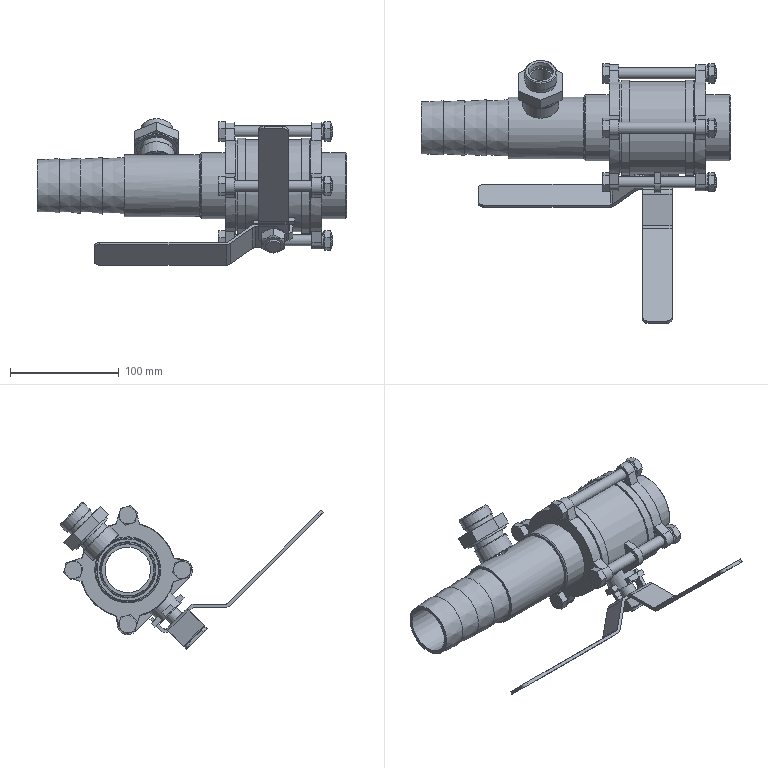Part | STEP file | COMPOUND | 23 solids | 365 faces | box 285 x 242.184 x 135.057 mm | volume 593050 mm3 | plane 232 | cylinder 95 | cone 37 | sphere 1 | commonest cylinder face diameters 10 x16 16 x8 6 x6 12 x6 10.001 x4 10.55 x4